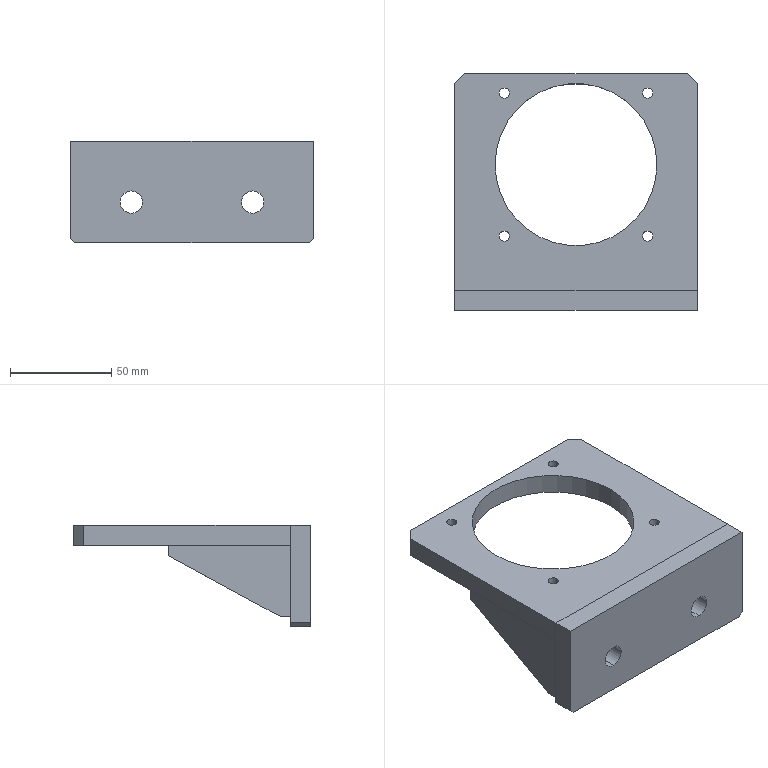Part | SolidWorks | features ICE 3, Chamfer 2, HoleWzd 2, Extrusion 1, MirrorSolid 1 | 4 solids | 44 faces | box 120 x 117 x 50 mm | volume 147908 mm3 | plane 30 | cylinder 14 | commonest cylinder face diameters 5 x8 11 x4 80 x2
STEP:
#1=CARTESIAN_POINT('',(-60.,5.,15.));
#2=VERTEX_POINT('',#1);
#3=CARTESIAN_POINT('',(-60.,65.,15.));
#4=VERTEX_POINT('',#3);
#5=CARTESIAN_POINT('',(-60.,5.,15.));
#6=DIRECTION('',(0.,1.,0.));
#7=VECTOR('',#6,1000.);
#8=LINE('',#5,#7);
#9=EDGE_CURVE('',#2,#4,#8,.T.);
#10=ORIENTED_EDGE('',*,*,#9,.F.);
#11=CARTESIAN_POINT('',(-55.,5.,15.));
#12=VERTEX_POINT('',#11);
#13=CARTESIAN_POINT('',(-55.,5.,15.));
#14=DIRECTION('',(-1.,0.,0.));
#15=VECTOR('',#14,1000.);
#16=LINE('',#13,#15);
#17=EDGE_CURVE('',#12,#2,#16,.T.);
#18=ORIENTED_EDGE('',*,*,#17,.F.);
#19=CARTESIAN_POINT('',(-55.,65.,15.));
#20=VERTEX_POINT('',#19);
#21=CARTESIAN_POINT('',(-55.,5.,15.));
#22=DIRECTION('',(0.,1.,0.));
#23=VECTOR('',#22,1000.);
#24=LINE('',#21,#23);
#25=EDGE_CURVE('',#12,#20,#24,.T.);
#26=ORIENTED_EDGE('',*,*,#25,.T.);
#27=CARTESIAN_POINT('',(-55.,65.,15.));
#28=DIRECTION('',(-1.,0.,0.));
#29=VECTOR('',#28,1000.);
#30=LINE('',#27,#29);
#31=EDGE_CURVE('',#20,#4,#30,.T.);
#32=ORIENTED_EDGE('',*,*,#31,.T.);
#33=EDGE_LOOP('',(#10,#18,#26,#32));
#34=FACE_OUTER_BOUND('',#33,.T.);
#35=CARTESIAN_POINT('',(-55.,5.,15.));
#36=DIRECTION('',(0.,0.,1.));
#37=DIRECTION('',(1.,0.,0.));
#38=AXIS2_PLACEMENT_3D('',#35,#36,#37);
#39=PLANE('',#38);
#40=ADVANCED_FACE('',(#34),#39,.T.);
#41=CARTESIAN_POINT('',(-60.,5.,-20.));
#42=VERTEX_POINT('',#41);
#43=CARTESIAN_POINT('',(-60.,5.,-20.));
#44=DIRECTION('',(0.,0.,1.));
#45=VECTOR('',#44,1000.);
#46=LINE('',#43,#45);
#47=EDGE_CURVE('',#42,#2,#46,.T.);
#48=ORIENTED_EDGE('',*,*,#47,.F.);
#49=CARTESIAN_POINT('',(-55.,5.,-20.));
#50=VERTEX_POINT('',#49);
#51=CARTESIAN_POINT('',(-55.,5.,-20.));
#52=DIRECTION('',(-1.,0.,0.));
#53=VECTOR('',#52,1000.);
#54=LINE('',#51,#53);
#55=EDGE_CURVE('',#50,#42,#54,.T.);
#56=ORIENTED_EDGE('',*,*,#55,.F.);
#57=CARTESIAN_POINT('',(-55.,5.,-20.));
#58=DIRECTION('',(0.,0.,1.));
#59=VECTOR('',#58,1000.);
#60=LINE('',#57,#59);
#61=EDGE_CURVE('',#50,#12,#60,.T.);
#62=ORIENTED_EDGE('',*,*,#61,.T.);
#63=ORIENTED_EDGE('',*,*,#17,.T.);
#64=EDGE_LOOP('',(#48,#56,#62,#63));
#65=FACE_OUTER_BOUND('',#64,.T.);
#66=CARTESIAN_POINT('',(-55.,5.,-20.));
#67=DIRECTION('',(0.,-1.,0.));
#68=DIRECTION('',(0.,0.,-1.));
#69=AXIS2_PLACEMENT_3D('',#66,#67,#68);
#70=PLANE('',#69);
#71=ADVANCED_FACE('',(#65),#70,.T.);
#72=CARTESIAN_POINT('',(-60.,10.,-20.));
#73=VERTEX_POINT('',#72);
#74=CARTESIAN_POINT('',(-60.,10.,-20.));
#75=DIRECTION('',(0.,-1.,0.));
#76=VECTOR('',#75,1000.);
#77=LINE('',#74,#76);
#78=EDGE_CURVE('',#73,#42,#77,.T.);
#79=ORIENTED_EDGE('',*,*,#78,.F.);
#80=CARTESIAN_POINT('',(-55.,10.,-20.));
#81=VERTEX_POINT('',#80);
#82=CARTESIAN_POINT('',(-55.,10.,-20.));
#83=DIRECTION('',(-1.,0.,0.));
#84=VECTOR('',#83,1000.);
#85=LINE('',#82,#84);
#86=EDGE_CURVE('',#81,#73,#85,.T.);
#87=ORIENTED_EDGE('',*,*,#86,.F.);
#88=CARTESIAN_POINT('',(-55.,10.,-20.));
#89=DIRECTION('',(0.,-1.,0.));
#90=VECTOR('',#89,1000.);
#91=LINE('',#88,#90);
#92=EDGE_CURVE('',#81,#50,#91,.T.);
#93=ORIENTED_EDGE('',*,*,#92,.T.);
#94=ORIENTED_EDGE('',*,*,#55,.T.);
#95=EDGE_LOOP('',(#79,#87,#93,#94));
#96=FACE_OUTER_BOUND('',#95,.T.);
#97=CARTESIAN_POINT('',(-55.,10.,-20.));
#98=DIRECTION('',(0.,0.,-1.));
#99=DIRECTION('',(-1.,0.,0.));
#100=AXIS2_PLACEMENT_3D('',#97,#98,#99);
#101=PLANE('',#100);
#102=ADVANCED_FACE('',(#96),#101,.T.);
#103=CARTESIAN_POINT('',(-60.,65.,10.));
#104=VERTEX_POINT('',#103);
#105=CARTESIAN_POINT('',(-60.,65.,10.));
#106=DIRECTION('',(0.,-0.8779,-0.4789));
#107=VECTOR('',#106,1000.);
#108=LINE('',#105,#107);
#109=EDGE_CURVE('',#104,#73,#108,.T.);
#110=ORIENTED_EDGE('',*,*,#109,.F.);
#111=CARTESIAN_POINT('',(-55.,65.,10.));
#112=VERTEX_POINT('',#111);
#113=CARTESIAN_POINT('',(-55.,65.,10.));
#114=DIRECTION('',(-1.,0.,0.));
#115=VECTOR('',#114,1000.);
#116=LINE('',#113,#115);
#117=EDGE_CURVE('',#112,#104,#116,.T.);
#118=ORIENTED_EDGE('',*,*,#117,.F.);
#119=CARTESIAN_POINT('',(-55.,65.,10.));
#120=DIRECTION('',(0.,-0.8779,-0.4789));
#121=VECTOR('',#120,1000.);
#122=LINE('',#119,#121);
#123=EDGE_CURVE('',#112,#81,#122,.T.);
#124=ORIENTED_EDGE('',*,*,#123,.T.);
#125=ORIENTED_EDGE('',*,*,#86,.T.);
#126=EDGE_LOOP('',(#110,#118,#124,#125));
#127=FACE_OUTER_BOUND('',#126,.T.);
#128=CARTESIAN_POINT('',(-55.,65.,10.));
#129=DIRECTION('',(0.,0.4789,-0.8779));
#130=DIRECTION('',(0.,0.8779,0.4789));
#131=AXIS2_PLACEMENT_3D('',#128,#129,#130);
#132=PLANE('',#131);
#133=ADVANCED_FACE('',(#127),#132,.T.);
#134=CARTESIAN_POINT('',(-60.,65.,15.));
#135=DIRECTION('',(0.,0.,-1.));
#136=VECTOR('',#135,1000.);
#137=LINE('',#134,#136);
#138=EDGE_CURVE('',#4,#104,#137,.T.);
#139=ORIENTED_EDGE('',*,*,#138,.F.);
#140=ORIENTED_EDGE('',*,*,#31,.F.);
#141=CARTESIAN_POINT('',(-55.,65.,15.));
#142=DIRECTION('',(0.,0.,-1.));
#143=VECTOR('',#142,1000.);
#144=LINE('',#141,#143);
#145=EDGE_CURVE('',#20,#112,#144,.T.);
#146=ORIENTED_EDGE('',*,*,#145,.T.);
#147=ORIENTED_EDGE('',*,*,#117,.T.);
#148=EDGE_LOOP('',(#139,#140,#146,#147));
#149=FACE_OUTER_BOUND('',#148,.T.);
#150=CARTESIAN_POINT('',(-55.,65.,15.));
#151=DIRECTION('',(0.,1.,0.));
#152=DIRECTION('',(0.,0.,1.));
#153=AXIS2_PLACEMENT_3D('',#150,#151,#152);
#154=PLANE('',#153);
#155=ADVANCED_FACE('',(#149),#154,.T.);
#156=ORIENTED_EDGE('',*,*,#25,.F.);
#157=ORIENTED_EDGE('',*,*,#61,.F.);
#158=ORIENTED_EDGE('',*,*,#92,.F.);
#159=ORIENTED_EDGE('',*,*,#123,.F.);
#160=ORIENTED_EDGE('',*,*,#145,.F.);
#161=EDGE_LOOP('',(#156,#157,#158,#159,#160));
#162=FACE_OUTER_BOUND('',#161,.T.);
#163=CARTESIAN_POINT('',(-55.,0.,0.));
#164=DIRECTION('',(-1.,0.,0.));
#165=DIRECTION('',(0.,0.,1.));
#166=AXIS2_PLACEMENT_3D('',#163,#164,#165);
#167=PLANE('',#166);
#168=ADVANCED_FACE('',(#162),#167,.F.);
#169=ORIENTED_EDGE('',*,*,#9,.T.);
#170=ORIENTED_EDGE('',*,*,#138,.T.);
#171=ORIENTED_EDGE('',*,*,#109,.T.);
#172=ORIENTED_EDGE('',*,*,#78,.T.);
#173=ORIENTED_EDGE('',*,*,#47,.T.);
#174=EDGE_LOOP('',(#169,#170,#171,#172,#173));
#175=FACE_OUTER_BOUND('',#174,.T.);
#176=CARTESIAN_POINT('',(-60.,0.,0.));
#177=DIRECTION('',(-1.,0.,0.));
#178=DIRECTION('',(0.,0.,1.));
#179=AXIS2_PLACEMENT_3D('',#176,#177,#178);
#180=PLANE('',#179);
#181=ADVANCED_FACE('',(#175),#180,.T.);
#182=CLOSED_SHELL('',(#40,#71,#102,#133,#155,#168,#181));
#183=MANIFOLD_SOLID_BREP('',#182);
#184=CARTESIAN_POINT('',(60.,5.,15.));
#185=VERTEX_POINT('',#184);
#186=CARTESIAN_POINT('',(60.,65.,15.));
#187=VERTEX_POINT('',#186);
#188=CARTESIAN_POINT('',(60.,5.,15.));
#189=DIRECTION('',(0.,1.,0.));
#190=VECTOR('',#189,1000.);
#191=LINE('',#188,#190);
#192=EDGE_CURVE('',#185,#187,#191,.T.);
#193=ORIENTED_EDGE('',*,*,#192,.T.);
#194=CARTESIAN_POINT('',(55.,65.,15.));
#195=VERTEX_POINT('',#194);
#196=CARTESIAN_POINT('',(55.,65.,15.));
#197=DIRECTION('',(1.,0.,0.));
#198=VECTOR('',#197,1000.);
#199=LINE('',#196,#198);
#200=EDGE_CURVE('',#195,#187,#199,.T.);
#201=ORIENTED_EDGE('',*,*,#200,.F.);
#202=CARTESIAN_POINT('',(55.,5.,15.));
#203=VERTEX_POINT('',#202);
#204=CARTESIAN_POINT('',(55.,5.,15.));
#205=DIRECTION('',(0.,1.,0.));
#206=VECTOR('',#205,1000.);
#207=LINE('',#204,#206);
#208=EDGE_CURVE('',#203,#195,#207,.T.);
#209=ORIENTED_EDGE('',*,*,#208,.F.);
#210=CARTESIAN_POINT('',(55.,5.,15.));
#211=DIRECTION('',(1.,0.,0.));
#212=VECTOR('',#211,1000.);
#213=LINE('',#210,#212);
#214=EDGE_CURVE('',#203,#185,#213,.T.);
#215=ORIENTED_EDGE('',*,*,#214,.T.);
#216=EDGE_LOOP('',(#193,#201,#209,#215));
#217=FACE_OUTER_BOUND('',#216,.T.);
#218=CARTESIAN_POINT('',(55.,5.,15.));
#219=DIRECTION('',(0.,0.,1.));
#220=DIRECTION('',(-1.,0.,0.));
#221=AXIS2_PLACEMENT_3D('',#218,#219,#220);
#222=PLANE('',#221);
#223=ADVANCED_FACE('',(#217),#222,.T.);
#224=CARTESIAN_POINT('',(60.,5.,-20.));
#225=VERTEX_POINT('',#224);
#226=CARTESIAN_POINT('',(60.,5.,-20.));
#227=DIRECTION('',(0.,0.,1.));
#228=VECTOR('',#227,1000.);
#229=LINE('',#226,#228);
#230=EDGE_CURVE('',#225,#185,#229,.T.);
#231=ORIENTED_EDGE('',*,*,#230,.T.);
#232=ORIENTED_EDGE('',*,*,#214,.F.);
#233=CARTESIAN_POINT('',(55.,5.,-20.));
#234=VERTEX_POINT('',#233);
#235=CARTESIAN_POINT('',(55.,5.,-20.));
#236=DIRECTION('',(0.,0.,1.));
#237=VECTOR('',#236,1000.);
#238=LINE('',#235,#237);
#239=EDGE_CURVE('',#234,#203,#238,.T.);
#240=ORIENTED_EDGE('',*,*,#239,.F.);
#241=CARTESIAN_POINT('',(55.,5.,-20.));
#242=DIRECTION('',(1.,0.,0.));
#243=VECTOR('',#242,1000.);
#244=LINE('',#241,#243);
#245=EDGE_CURVE('',#234,#225,#244,.T.);
#246=ORIENTED_EDGE('',*,*,#245,.T.);
#247=EDGE_LOOP('',(#231,#232,#240,#246));
#248=FACE_OUTER_BOUND('',#247,.T.);
#249=CARTESIAN_POINT('',(55.,5.,-20.));
#250=DIRECTION('',(0.,-1.,0.));
#251=DIRECTION('',(0.,0.,-1.));
#252=AXIS2_PLACEMENT_3D('',#249,#250,#251);
#253=PLANE('',#252);
#254=ADVANCED_FACE('',(#248),#253,.T.);
#255=CARTESIAN_POINT('',(60.,10.,-20.));
#256=VERTEX_POINT('',#255);
#257=CARTESIAN_POINT('',(60.,10.,-20.));
#258=DIRECTION('',(0.,-1.,0.));
#259=VECTOR('',#258,1000.);
#260=LINE('',#257,#259);
#261=EDGE_CURVE('',#256,#225,#260,.T.);
#262=ORIENTED_EDGE('',*,*,#261,.T.);
#263=ORIENTED_EDGE('',*,*,#245,.F.);
#264=CARTESIAN_POINT('',(55.,10.,-20.));
#265=VERTEX_POINT('',#264);
#266=CARTESIAN_POINT('',(55.,10.,-20.));
#267=DIRECTION('',(0.,-1.,0.));
#268=VECTOR('',#267,1000.);
#269=LINE('',#266,#268);
#270=EDGE_CURVE('',#265,#234,#269,.T.);
#271=ORIENTED_EDGE('',*,*,#270,.F.);
#272=CARTESIAN_POINT('',(55.,10.,-20.));
#273=DIRECTION('',(1.,0.,0.));
#274=VECTOR('',#273,1000.);
#275=LINE('',#272,#274);
#276=EDGE_CURVE('',#265,#256,#275,.T.);
#277=ORIENTED_EDGE('',*,*,#276,.T.);
#278=EDGE_LOOP('',(#262,#263,#271,#277));
#279=FACE_OUTER_BOUND('',#278,.T.);
#280=CARTESIAN_POINT('',(55.,10.,-20.));
#281=DIRECTION('',(0.,0.,-1.));
#282=DIRECTION('',(1.,0.,0.));
#283=AXIS2_PLACEMENT_3D('',#280,#281,#282);
#284=PLANE('',#283);
#285=ADVANCED_FACE('',(#279),#284,.T.);
#286=CARTESIAN_POINT('',(60.,65.,10.));
#287=VERTEX_POINT('',#286);
#288=CARTESIAN_POINT('',(60.,65.,10.));
#289=DIRECTION('',(0.,-0.8779,-0.4789));
#290=VECTOR('',#289,1000.);
#291=LINE('',#288,#290);
#292=EDGE_CURVE('',#287,#256,#291,.T.);
#293=ORIENTED_EDGE('',*,*,#292,.T.);
#294=ORIENTED_EDGE('',*,*,#276,.F.);
#295=CARTESIAN_POINT('',(55.,65.,10.));
#296=VERTEX_POINT('',#295);
#297=CARTESIAN_POINT('',(55.,65.,10.));
#298=DIRECTION('',(0.,-0.8779,-0.4789));
#299=VECTOR('',#298,1000.);
#300=LINE('',#297,#299);
#301=EDGE_CURVE('',#296,#265,#300,.T.);
#302=ORIENTED_EDGE('',*,*,#301,.F.);
#303=CARTESIAN_POINT('',(55.,65.,10.));
#304=DIRECTION('',(1.,0.,0.));
#305=VECTOR('',#304,1000.);
#306=LINE('',#303,#305);
#307=EDGE_CURVE('',#296,#287,#306,.T.);
#308=ORIENTED_EDGE('',*,*,#307,.T.);
#309=EDGE_LOOP('',(#293,#294,#302,#308));
#310=FACE_OUTER_BOUND('',#309,.T.);
#311=CARTESIAN_POINT('',(55.,65.,10.));
#312=DIRECTION('',(0.,0.4789,-0.8779));
#313=DIRECTION('',(0.,0.8779,0.4789));
#314=AXIS2_PLACEMENT_3D('',#311,#312,#313);
#315=PLANE('',#314);
#316=ADVANCED_FACE('',(#310),#315,.T.);
#317=CARTESIAN_POINT('',(60.,65.,15.));
#318=DIRECTION('',(0.,0.,-1.));
#319=VECTOR('',#318,1000.);
#320=LINE('',#317,#319);
#321=EDGE_CURVE('',#187,#287,#320,.T.);
#322=ORIENTED_EDGE('',*,*,#321,.T.);
#323=ORIENTED_EDGE('',*,*,#307,.F.);
#324=CARTESIAN_POINT('',(55.,65.,15.));
#325=DIRECTION('',(0.,0.,-1.));
#326=VECTOR('',#325,1000.);
#327=LINE('',#324,#326);
#328=EDGE_CURVE('',#195,#296,#327,.T.);
#329=ORIENTED_EDGE('',*,*,#328,.F.);
#330=ORIENTED_EDGE('',*,*,#200,.T.);
#331=EDGE_LOOP('',(#322,#323,#329,#330));
#332=FACE_OUTER_BOUND('',#331,.T.);
#333=CARTESIAN_POINT('',(55.,65.,15.));
#334=DIRECTION('',(0.,1.,0.));
#335=DIRECTION('',(0.,0.,1.));
#336=AXIS2_PLACEMENT_3D('',#333,#334,#335);
#337=PLANE('',#336);
#338=ADVANCED_FACE('',(#332),#337,.T.);
#339=ORIENTED_EDGE('',*,*,#208,.T.);
#340=ORIENTED_EDGE('',*,*,#328,.T.);
#341=ORIENTED_EDGE('',*,*,#301,.T.);
#342=ORIENTED_EDGE('',*,*,#270,.T.);
#343=ORIENTED_EDGE('',*,*,#239,.T.);
#344=EDGE_LOOP('',(#339,#340,#341,#342,#343));
#345=FACE_OUTER_BOUND('',#344,.T.);
#346=CARTESIAN_POINT('',(55.,0.,0.));
#347=DIRECTION('',(1.,0.,0.));
#348=DIRECTION('',(0.,0.,1.));
#349=AXIS2_PLACEMENT_3D('',#346,#347,#348);
#350=PLANE('',#349);
#351=ADVANCED_FACE('',(#345),#350,.F.);
#352=ORIENTED_EDGE('',*,*,#192,.F.);
#353=ORIENTED_EDGE('',*,*,#230,.F.);
#354=ORIENTED_EDGE('',*,*,#261,.F.);
#355=ORIENTED_EDGE('',*,*,#292,.F.);
#356=ORIENTED_EDGE('',*,*,#321,.F.);
#357=EDGE_LOOP('',(#352,#353,#354,#355,#356));
#358=FACE_OUTER_BOUND('',#357,.T.);
#359=CARTESIAN_POINT('',(60.,0.,0.));
#360=DIRECTION('',(1.,0.,0.));
#361=DIRECTION('',(0.,0.,1.));
#362=AXIS2_PLACEMENT_3D('',#359,#360,#361);
#363=PLANE('',#362);
#364=ADVANCED_FACE('',(#358),#363,.T.);
#365=CLOSED_SHELL('',(#223,#254,#285,#316,#338,#351,#364));
#366=MANIFOLD_SOLID_BREP('',#365);
#367=CARTESIAN_POINT('',(30.,-5.,-10.5));
#368=VERTEX_POINT('',#367);
#369=CARTESIAN_POINT('',(30.,-5.,0.5));
#370=VERTEX_POINT('',#369);
#371=CARTESIAN_POINT('',(30.,-5.,-5.));
#372=DIRECTION('',(0.,1.,0.));
#373=DIRECTION('',(0.,0.,1.));
#374=AXIS2_PLACEMENT_3D('',#371,#372,#373);
#375=CIRCLE('',#374,5.5);
#376=EDGE_CURVE('',#368,#370,#375,.T.);
#377=ORIENTED_EDGE('',*,*,#376,.F.);
#378=CARTESIAN_POINT('',(30.,5.,-10.5));
#379=VERTEX_POINT('',#378);
#380=CARTESIAN_POINT('',(30.,5.,-10.5));
#381=DIRECTION('',(0.,1.,0.));
#382=VECTOR('',#381,1000.);
#383=LINE('',#380,#382);
#384=EDGE_CURVE('',#368,#379,#383,.T.);
#385=ORIENTED_EDGE('',*,*,#384,.T.);
#386=CARTESIAN_POINT('',(30.,5.,0.5));
#387=VERTEX_POINT('',#386);
#388=CARTESIAN_POINT('',(30.,5.,-5.));
#389=DIRECTION('',(0.,1.,0.));
#390=DIRECTION('',(0.,0.,1.));
#391=AXIS2_PLACEMENT_3D('',#388,#389,#390);
#392=CIRCLE('',#391,5.5);
#393=EDGE_CURVE('',#379,#387,#392,.T.);
#394=ORIENTED_EDGE('',*,*,#393,.T.);
#395=CARTESIAN_POINT('',(30.,5.,0.5));
#396=DIRECTION('',(0.,1.,0.));
#397=VECTOR('',#396,1000.);
#398=LINE('',#395,#397);
#399=EDGE_CURVE('',#370,#387,#398,.T.);
#400=ORIENTED_EDGE('',*,*,#399,.F.);
#401=EDGE_LOOP('',(#377,#385,#394,#400));
#402=FACE_OUTER_BOUND('',#401,.T.);
#403=CARTESIAN_POINT('',(30.,5.,-5.));
#404=DIRECTION('',(0.,1.,0.));
#405=DIRECTION('',(0.,0.,1.));
#406=AXIS2_PLACEMENT_3D('',#403,#404,#405);
#407=CYLINDRICAL_SURFACE('',#406,5.5);
#408=ADVANCED_FACE('',(#402),#407,.F.);
#409=CARTESIAN_POINT('',(-30.,-5.,-10.5));
#410=VERTEX_POINT('',#409);
#411=CARTESIAN_POINT('',(-30.,-5.,0.5));
#412=VERTEX_POINT('',#411);
#413=CARTESIAN_POINT('',(-30.,-5.,-5.));
#414=DIRECTION('',(0.,1.,0.));
#415=DIRECTION('',(0.,0.,1.));
#416=AXIS2_PLACEMENT_3D('',#413,#414,#415);
#417=CIRCLE('',#416,5.5);
#418=EDGE_CURVE('',#410,#412,#417,.T.);
#419=ORIENTED_EDGE('',*,*,#418,.F.);
#420=CARTESIAN_POINT('',(-30.,5.,-10.5));
#421=VERTEX_POINT('',#420);
#422=CARTESIAN_POINT('',(-30.,5.,-10.5));
#423=DIRECTION('',(0.,1.,0.));
#424=VECTOR('',#423,1000.);
#425=LINE('',#422,#424);
#426=EDGE_CURVE('',#410,#421,#425,.T.);
#427=ORIENTED_EDGE('',*,*,#426,.T.);
#428=CARTESIAN_POINT('',(-30.,5.,0.5));
#429=VERTEX_POINT('',#428);
#430=CARTESIAN_POINT('',(-30.,5.,-5.));
#431=DIRECTION('',(0.,1.,0.));
#432=DIRECTION('',(0.,0.,1.));
#433=AXIS2_PLACEMENT_3D('',#430,#431,#432);
#434=CIRCLE('',#433,5.5);
#435=EDGE_CURVE('',#421,#429,#434,.T.);
#436=ORIENTED_EDGE('',*,*,#435,.T.);
#437=CARTESIAN_POINT('',(-30.,5.,0.5));
#438=DIRECTION('',(0.,1.,0.));
#439=VECTOR('',#438,1000.);
#440=LINE('',#437,#439);
#441=EDGE_CURVE('',#412,#429,#440,.T.);
#442=ORIENTED_EDGE('',*,*,#441,.F.);
#443=EDGE_LOOP('',(#419,#427,#436,#442));
#444=FACE_OUTER_BOUND('',#443,.T.);
#445=CARTESIAN_POINT('',(-30.,5.,-5.));
#446=DIRECTION('',(0.,1.,0.));
#447=DIRECTION('',(0.,0.,1.));
#448=AXIS2_PLACEMENT_3D('',#445,#446,#447);
#449=CYLINDRICAL_SURFACE('',#448,5.5);
#450=ADVANCED_FACE('',(#444),#449,.F.);
#451=CARTESIAN_POINT('',(60.,-5.,25.));
#452=VERTEX_POINT('',#451);
#453=CARTESIAN_POINT('',(60.,-5.,-23.));
#454=VERTEX_POINT('',#453);
#455=CARTESIAN_POINT('',(60.,-5.,25.));
#456=DIRECTION('',(0.,0.,-1.));
#457=VECTOR('',#456,1000.);
#458=LINE('',#455,#457);
#459=EDGE_CURVE('',#452,#454,#458,.T.);
#460=ORIENTED_EDGE('',*,*,#459,.T.);
#461=CARTESIAN_POINT('',(60.,5.,-23.));
#462=VERTEX_POINT('',#461);
#463=CARTESIAN_POINT('',(60.,5.,-23.));
#464=DIRECTION('',(0.,1.,0.));
#465=VECTOR('',#464,1000.);
#466=LINE('',#463,#465);
#467=EDGE_CURVE('',#454,#462,#466,.T.);
#468=ORIENTED_EDGE('',*,*,#467,.T.);
#469=CARTESIAN_POINT('',(60.,5.,25.));
#470=VERTEX_POINT('',#469);
#471=CARTESIAN_POINT('',(60.,5.,25.));
#472=DIRECTION('',(0.,0.,-1.));
#473=VECTOR('',#472,1000.);
#474=LINE('',#471,#473);
#475=EDGE_CURVE('',#470,#462,#474,.T.);
#476=ORIENTED_EDGE('',*,*,#475,.F.);
#477=CARTESIAN_POINT('',(60.,5.,25.));
#478=DIRECTION('',(0.,-1.,0.));
#479=VECTOR('',#478,1000.);
#480=LINE('',#477,#479);
#481=EDGE_CURVE('',#470,#452,#480,.T.);
#482=ORIENTED_EDGE('',*,*,#481,.T.);
#483=EDGE_LOOP('',(#460,#468,#476,#482));
#484=FACE_OUTER_BOUND('',#483,.T.);
#485=CARTESIAN_POINT('',(60.,5.,25.));
#486=DIRECTION('',(-1.,0.,0.));
#487=DIRECTION('',(0.,0.,1.));
#488=AXIS2_PLACEMENT_3D('',#485,#486,#487);
#489=PLANE('',#488);
#490=ADVANCED_FACE('',(#484),#489,.F.);
#491=CARTESIAN_POINT('',(58.,-5.,-25.));
#492=VERTEX_POINT('',#491);
#493=CARTESIAN_POINT('',(-58.,-5.,-25.));
#494=VERTEX_POINT('',#493);
#495=CARTESIAN_POINT('',(-60.,-5.,-25.));
#496=DIRECTION('',(-1.,0.,0.));
#497=VECTOR('',#496,1000.);
#498=LINE('',#495,#497);
#499=EDGE_CURVE('',#492,#494,#498,.T.);
#500=ORIENTED_EDGE('',*,*,#499,.T.);
#501=CARTESIAN_POINT('',(-58.,5.,-25.));
#502=VERTEX_POINT('',#501);
#503=CARTESIAN_POINT('',(-58.,5.,-25.));
#504=DIRECTION('',(0.,1.,0.));
#505=VECTOR('',#504,1000.);
#506=LINE('',#503,#505);
#507=EDGE_CURVE('',#494,#502,#506,.T.);
#508=ORIENTED_EDGE('',*,*,#507,.T.);
#509=CARTESIAN_POINT('',(58.,5.,-25.));
#510=VERTEX_POINT('',#509);
#511=CARTESIAN_POINT('',(-60.,5.,-25.));
#512=DIRECTION('',(-1.,0.,0.));
#513=VECTOR('',#512,1000.);
#514=LINE('',#511,#513);
#515=EDGE_CURVE('',#510,#502,#514,.T.);
#516=ORIENTED_EDGE('',*,*,#515,.F.);
#517=CARTESIAN_POINT('',(58.,5.,-25.));
#518=DIRECTION('',(0.,-1.,0.));
#519=VECTOR('',#518,1000.);
#520=LINE('',#517,#519);
#521=EDGE_CURVE('',#510,#492,#520,.T.);
#522=ORIENTED_EDGE('',*,*,#521,.T.);
#523=EDGE_LOOP('',(#500,#508,#516,#522));
#524=FACE_OUTER_BOUND('',#523,.T.);
#525=CARTESIAN_POINT('',(-60.,5.,-25.));
#526=DIRECTION('',(0.,0.,1.));
#527=DIRECTION('',(1.,0.,0.));
#528=AXIS2_PLACEMENT_3D('',#525,#526,#527);
#529=PLANE('',#528);
#530=ADVANCED_FACE('',(#524),#529,.F.);
#531=CARTESIAN_POINT('',(-60.,5.,-23.));
#532=VERTEX_POINT('',#531);
#533=CARTESIAN_POINT('',(-60.,5.,25.));
#534=VERTEX_POINT('',#533);
#535=CARTESIAN_POINT('',(-60.,5.,25.));
#536=DIRECTION('',(0.,0.,1.));
#537=VECTOR('',#536,1000.);
#538=LINE('',#535,#537);
#539=EDGE_CURVE('',#532,#534,#538,.T.);
#540=ORIENTED_EDGE('',*,*,#539,.F.);
#541=CARTESIAN_POINT('',(-60.,-5.,-23.));
#542=VERTEX_POINT('',#541);
#543=CARTESIAN_POINT('',(-60.,5.,-23.));
#544=DIRECTION('',(0.,-1.,0.));
#545=VECTOR('',#544,1000.);
#546=LINE('',#543,#545);
#547=EDGE_CURVE('',#532,#542,#546,.T.);
#548=ORIENTED_EDGE('',*,*,#547,.T.);
#549=CARTESIAN_POINT('',(-60.,-5.,25.));
#550=VERTEX_POINT('',#549);
#551=CARTESIAN_POINT('',(-60.,-5.,25.));
#552=DIRECTION('',(0.,0.,1.));
#553=VECTOR('',#552,1000.);
#554=LINE('',#551,#553);
#555=EDGE_CURVE('',#542,#550,#554,.T.);
#556=ORIENTED_EDGE('',*,*,#555,.T.);
#557=CARTESIAN_POINT('',(-60.,5.,25.));
#558=DIRECTION('',(0.,-1.,0.));
#559=VECTOR('',#558,1000.);
#560=LINE('',#557,#559);
#561=EDGE_CURVE('',#534,#550,#560,.T.);
#562=ORIENTED_EDGE('',*,*,#561,.F.);
#563=EDGE_LOOP('',(#540,#548,#556,#562));
#564=FACE_OUTER_BOUND('',#563,.T.);
#565=CARTESIAN_POINT('',(-60.,5.,25.));
#566=DIRECTION('',(1.,0.,0.));
#567=DIRECTION('',(0.,0.,-1.));
#568=AXIS2_PLACEMENT_3D('',#565,#566,#567);
#569=PLANE('',#568);
#570=ADVANCED_FACE('',(#564),#569,.F.);
#571=CARTESIAN_POINT('',(-60.,-5.,25.));
#572=DIRECTION('',(1.,0.,0.));
#573=VECTOR('',#572,1000.);
#574=LINE('',#571,#573);
#575=EDGE_CURVE('',#550,#452,#574,.T.);
#576=ORIENTED_EDGE('',*,*,#575,.T.);
#577=ORIENTED_EDGE('',*,*,#481,.F.);
#578=CARTESIAN_POINT('',(-60.,5.,25.));
#579=DIRECTION('',(1.,0.,0.));
#580=VECTOR('',#579,1000.);
#581=LINE('',#578,#580);
#582=EDGE_CURVE('',#534,#470,#581,.T.);
#583=ORIENTED_EDGE('',*,*,#582,.F.);
#584=ORIENTED_EDGE('',*,*,#561,.T.);
#585=EDGE_LOOP('',(#576,#577,#583,#584));
#586=FACE_OUTER_BOUND('',#585,.T.);
#587=CARTESIAN_POINT('',(-60.,5.,25.));
#588=DIRECTION('',(0.,0.,-1.));
#589=DIRECTION('',(-1.,0.,0.));
#590=AXIS2_PLACEMENT_3D('',#587,#588,#589);
#591=PLANE('',#590);
#592=ADVANCED_FACE('',(#586),#591,.F.);
#593=CARTESIAN_POINT('',(30.,5.,-5.));
#594=DIRECTION('',(0.,1.,0.));
#595=DIRECTION('',(0.,0.,1.));
#596=AXIS2_PLACEMENT_3D('',#593,#594,#595);
#597=CIRCLE('',#596,5.5);
#598=EDGE_CURVE('',#387,#379,#597,.T.);
#599=ORIENTED_EDGE('',*,*,#598,.F.);
#600=ORIENTED_EDGE('',*,*,#393,.F.);
#601=EDGE_LOOP('',(#599,#600));
#602=FACE_BOUND('',#601,.T.);
#603=CARTESIAN_POINT('',(-30.,5.,-5.));
#604=DIRECTION('',(0.,1.,0.));
#605=DIRECTION('',(0.,0.,1.));
#606=AXIS2_PLACEMENT_3D('',#603,#604,#605);
#607=CIRCLE('',#606,5.5);
#608=EDGE_CURVE('',#429,#421,#607,.T.);
#609=ORIENTED_EDGE('',*,*,#608,.F.);
#610=ORIENTED_EDGE('',*,*,#435,.F.);
#611=EDGE_LOOP('',(#609,#610));
#612=FACE_BOUND('',#611,.T.);
#613=ORIENTED_EDGE('',*,*,#515,.T.);
#614=CARTESIAN_POINT('',(-60.,5.,-23.));
#615=DIRECTION('',(-0.7071,0.,0.7071));
#616=VECTOR('',#615,1000.);
#617=LINE('',#614,#616);
#618=EDGE_CURVE('',#502,#532,#617,.T.);
#619=ORIENTED_EDGE('',*,*,#618,.T.);
#620=ORIENTED_EDGE('',*,*,#539,.T.);
#621=ORIENTED_EDGE('',*,*,#582,.T.);
#622=ORIENTED_EDGE('',*,*,#475,.T.);
#623=CARTESIAN_POINT('',(58.,5.,-25.));
#624=DIRECTION('',(-0.7071,0.,-0.7071));
#625=VECTOR('',#624,1000.);
#626=LINE('',#623,#625);
#627=EDGE_CURVE('',#462,#510,#626,.T.);
#628=ORIENTED_EDGE('',*,*,#627,.T.);
#629=EDGE_LOOP('',(#613,#619,#620,#621,#622,#628));
#630=FACE_OUTER_BOUND('',#629,.T.);
#631=CARTESIAN_POINT('',(0.,5.,0.));
#632=DIRECTION('',(0.,-1.,0.));
#633=DIRECTION('',(0.,0.,-1.));
#634=AXIS2_PLACEMENT_3D('',#631,#632,#633);
#635=PLANE('',#634);
#636=ADVANCED_FACE('',(#602,#612,#630),#635,.F.);
#637=CARTESIAN_POINT('',(30.,-5.,-5.));
#638=DIRECTION('',(0.,1.,0.));
#639=DIRECTION('',(0.,0.,1.));
#640=AXIS2_PLACEMENT_3D('',#637,#638,#639);
#641=CIRCLE('',#640,5.5);
#642=EDGE_CURVE('',#370,#368,#641,.T.);
#643=ORIENTED_EDGE('',*,*,#642,.T.);
#644=ORIENTED_EDGE('',*,*,#376,.T.);
#645=EDGE_LOOP('',(#643,#644));
#646=FACE_BOUND('',#645,.T.);
#647=CARTESIAN_POINT('',(-30.,-5.,-5.));
#648=DIRECTION('',(0.,1.,0.));
#649=DIRECTION('',(0.,0.,1.));
#650=AXIS2_PLACEMENT_3D('',#647,#648,#649);
#651=CIRCLE('',#650,5.5);
#652=EDGE_CURVE('',#412,#410,#651,.T.);
#653=ORIENTED_EDGE('',*,*,#652,.T.);
#654=ORIENTED_EDGE('',*,*,#418,.T.);
#655=EDGE_LOOP('',(#653,#654));
#656=FACE_BOUND('',#655,.T.);
#657=ORIENTED_EDGE('',*,*,#555,.F.);
#658=CARTESIAN_POINT('',(-41.5,-5.,-41.5));
#659=DIRECTION('',(0.7071,0.,-0.7071));
#660=VECTOR('',#659,1000.);
#661=LINE('',#658,#660);
#662=EDGE_CURVE('',#542,#494,#661,.T.);
#663=ORIENTED_EDGE('',*,*,#662,.T.);
#664=ORIENTED_EDGE('',*,*,#499,.F.);
#665=CARTESIAN_POINT('',(41.5,-5.,-41.5));
#666=DIRECTION('',(0.7071,0.,0.7071));
#667=VECTOR('',#666,1000.);
#668=LINE('',#665,#667);
#669=EDGE_CURVE('',#492,#454,#668,.T.);
#670=ORIENTED_EDGE('',*,*,#669,.T.);
#671=ORIENTED_EDGE('',*,*,#459,.F.);
#672=ORIENTED_EDGE('',*,*,#575,.F.);
#673=EDGE_LOOP('',(#657,#663,#664,#670,#671,#672));
#674=FACE_OUTER_BOUND('',#673,.T.);
#675=CARTESIAN_POINT('',(0.,-5.,0.));
#676=DIRECTION('',(0.,-1.,0.));
#677=DIRECTION('',(0.,0.,-1.));
#678=AXIS2_PLACEMENT_3D('',#675,#676,#677);
#679=PLANE('',#678);
#680=ADVANCED_FACE('',(#646,#656,#674),#679,.T.);
#681=ORIENTED_EDGE('',*,*,#618,.F.);
#682=ORIENTED_EDGE('',*,*,#507,.F.);
#683=ORIENTED_EDGE('',*,*,#662,.F.);
#684=ORIENTED_EDGE('',*,*,#547,.F.);
#685=EDGE_LOOP('',(#681,#682,#683,#684));
#686=FACE_OUTER_BOUND('',#685,.T.);
#687=CARTESIAN_POINT('',(-60.,5.,-23.));
#688=DIRECTION('',(0.7071,0.,0.7071));
#689=DIRECTION('',(0.,-1.,0.));
#690=AXIS2_PLACEMENT_3D('',#687,#688,#689);
#691=PLANE('',#690);
#692=ADVANCED_FACE('',(#686),#691,.F.);
#693=ORIENTED_EDGE('',*,*,#627,.F.);
#694=ORIENTED_EDGE('',*,*,#467,.F.);
#695=ORIENTED_EDGE('',*,*,#669,.F.);
#696=ORIENTED_EDGE('',*,*,#521,.F.);
#697=EDGE_LOOP('',(#693,#694,#695,#696));
#698=FACE_OUTER_BOUND('',#697,.T.);
#699=CARTESIAN_POINT('',(58.,5.,-25.));
#700=DIRECTION('',(-0.7071,0.,0.7071));
#701=DIRECTION('',(0.,-1.,0.));
#702=AXIS2_PLACEMENT_3D('',#699,#700,#701);
#703=PLANE('',#702);
#704=ADVANCED_FACE('',(#698),#703,.F.);
#705=ORIENTED_EDGE('',*,*,#426,.F.);
#706=ORIENTED_EDGE('',*,*,#652,.F.);
#707=ORIENTED_EDGE('',*,*,#441,.T.);
#708=ORIENTED_EDGE('',*,*,#608,.T.);
#709=EDGE_LOOP('',(#705,#706,#707,#708));
#710=FACE_OUTER_BOUND('',#709,.T.);
#711=CARTESIAN_POINT('',(-30.,5.,-5.));
#712=DIRECTION('',(0.,1.,0.));
#713=DIRECTION('',(0.,0.,1.));
#714=AXIS2_PLACEMENT_3D('',#711,#712,#713);
#715=CYLINDRICAL_SURFACE('',#714,5.5);
#716=ADVANCED_FACE('',(#710),#715,.F.);
#717=ORIENTED_EDGE('',*,*,#384,.F.);
#718=ORIENTED_EDGE('',*,*,#642,.F.);
#719=ORIENTED_EDGE('',*,*,#399,.T.);
#720=ORIENTED_EDGE('',*,*,#598,.T.);
#721=EDGE_LOOP('',(#717,#718,#719,#720));
#722=FACE_OUTER_BOUND('',#721,.T.);
#723=CARTESIAN_POINT('',(30.,5.,-5.));
#724=DIRECTION('',(0.,1.,0.));
#725=DIRECTION('',(0.,0.,1.));
#726=AXIS2_PLACEMENT_3D('',#723,#724,#725);
#727=CYLINDRICAL_SURFACE('',#726,5.5);
#728=ADVANCED_FACE('',(#722),#727,.F.);
#729=CLOSED_SHELL('',(#408,#450,#490,#530,#570,#592,#636,#680,#692,#704,#716,#728));
#730=MANIFOLD_SOLID_BREP('',#729);
#731=CARTESIAN_POINT('',(-37.855,102.355,15.));
#732=VERTEX_POINT('',#731);
#733=CARTESIAN_POINT('',(-32.855,102.355,15.));
#734=VERTEX_POINT('',#733);
#735=CARTESIAN_POINT('',(-35.355,102.355,15.));
#736=DIRECTION('',(0.,0.,1.));
#737=DIRECTION('',(1.,0.,0.));
#738=AXIS2_PLACEMENT_3D('',#735,#736,#737);
#739=CIRCLE('',#738,2.5);
#740=EDGE_CURVE('',#732,#734,#739,.T.);
#741=ORIENTED_EDGE('',*,*,#740,.F.);
#742=CARTESIAN_POINT('',(-37.855,102.355,25.));
#743=VERTEX_POINT('',#742);
#744=CARTESIAN_POINT('',(-37.855,102.355,25.));
#745=DIRECTION('',(0.,0.,1.));
#746=VECTOR('',#745,1000.);
#747=LINE('',#744,#746);
#748=EDGE_CURVE('',#732,#743,#747,.T.);
#749=ORIENTED_EDGE('',*,*,#748,.T.);
#750=CARTESIAN_POINT('',(-32.855,102.355,25.));
#751=VERTEX_POINT('',#750);
#752=CARTESIAN_POINT('',(-35.355,102.355,25.));
#753=DIRECTION('',(0.,0.,1.));
#754=DIRECTION('',(1.,0.,0.));
#755=AXIS2_PLACEMENT_3D('',#752,#753,#754);
#756=CIRCLE('',#755,2.5);
#757=EDGE_CURVE('',#743,#751,#756,.T.);
#758=ORIENTED_EDGE('',*,*,#757,.T.);
#759=CARTESIAN_POINT('',(-32.855,102.355,25.));
#760=DIRECTION('',(0.,0.,1.));
#761=VECTOR('',#760,1000.);
#762=LINE('',#759,#761);
#763=EDGE_CURVE('',#734,#751,#762,.T.);
#764=ORIENTED_EDGE('',*,*,#763,.F.);
#765=EDGE_LOOP('',(#741,#749,#758,#764));
#766=FACE_OUTER_BOUND('',#765,.T.);
#767=CARTESIAN_POINT('',(-35.355,102.355,25.));
#768=DIRECTION('',(0.,0.,1.));
#769=DIRECTION('',(1.,0.,0.));
#770=AXIS2_PLACEMENT_3D('',#767,#768,#769);
#771=CYLINDRICAL_SURFACE('',#770,2.5);
#772=ADVANCED_FACE('',(#766),#771,.F.);
#773=CARTESIAN_POINT('',(32.855,102.355,15.));
#774=VERTEX_POINT('',#773);
#775=CARTESIAN_POINT('',(37.855,102.355,15.));
#776=VERTEX_POINT('',#775);
#777=CARTESIAN_POINT('',(35.355,102.355,15.));
#778=DIRECTION('',(0.,0.,1.));
#779=DIRECTION('',(1.,0.,0.));
#780=AXIS2_PLACEMENT_3D('',#777,#778,#779);
#781=CIRCLE('',#780,2.5);
#782=EDGE_CURVE('',#774,#776,#781,.T.);
#783=ORIENTED_EDGE('',*,*,#782,.F.);
#784=CARTESIAN_POINT('',(32.855,102.355,25.));
#785=VERTEX_POINT('',#784);
#786=CARTESIAN_POINT('',(32.855,102.355,25.));
#787=DIRECTION('',(0.,0.,1.));
#788=VECTOR('',#787,1000.);
#789=LINE('',#786,#788);
#790=EDGE_CURVE('',#774,#785,#789,.T.);
#791=ORIENTED_EDGE('',*,*,#790,.T.);
#792=CARTESIAN_POINT('',(37.855,102.355,25.));
#793=VERTEX_POINT('',#792);
#794=CARTESIAN_POINT('',(35.355,102.355,25.));
#795=DIRECTION('',(0.,0.,1.));
#796=DIRECTION('',(1.,0.,0.));
#797=AXIS2_PLACEMENT_3D('',#794,#795,#796);
#798=CIRCLE('',#797,2.5);
#799=EDGE_CURVE('',#785,#793,#798,.T.);
#800=ORIENTED_EDGE('',*,*,#799,.T.);
#801=CARTESIAN_POINT('',(37.855,102.355,25.));
#802=DIRECTION('',(0.,0.,1.));
#803=VECTOR('',#802,1000.);
#804=LINE('',#801,#803);
#805=EDGE_CURVE('',#776,#793,#804,.T.);
#806=ORIENTED_EDGE('',*,*,#805,.F.);
#807=EDGE_LOOP('',(#783,#791,#800,#806));
#808=FACE_OUTER_BOUND('',#807,.T.);
#809=CARTESIAN_POINT('',(35.355,102.355,25.));
#810=DIRECTION('',(0.,0.,1.));
#811=DIRECTION('',(1.,0.,0.));
#812=AXIS2_PLACEMENT_3D('',#809,#810,#811);
#813=CYLINDRICAL_SURFACE('',#812,2.5);
#814=ADVANCED_FACE('',(#808),#813,.F.);
#815=CARTESIAN_POINT('',(32.855,31.645,15.));
#816=VERTEX_POINT('',#815);
#817=CARTESIAN_POINT('',(37.855,31.645,15.));
#818=VERTEX_POINT('',#817);
#819=CARTESIAN_POINT('',(35.355,31.645,15.));
#820=DIRECTION('',(0.,0.,1.));
#821=DIRECTION('',(1.,0.,0.));
#822=AXIS2_PLACEMENT_3D('',#819,#820,#821);
#823=CIRCLE('',#822,2.5);
#824=EDGE_CURVE('',#816,#818,#823,.T.);
#825=ORIENTED_EDGE('',*,*,#824,.F.);
#826=CARTESIAN_POINT('',(32.855,31.645,25.));
#827=VERTEX_POINT('',#826);
#828=CARTESIAN_POINT('',(32.855,31.645,25.));
#829=DIRECTION('',(0.,0.,1.));
#830=VECTOR('',#829,1000.);
#831=LINE('',#828,#830);
#832=EDGE_CURVE('',#816,#827,#831,.T.);
#833=ORIENTED_EDGE('',*,*,#832,.T.);
#834=CARTESIAN_POINT('',(37.855,31.645,25.));
#835=VERTEX_POINT('',#834);
#836=CARTESIAN_POINT('',(35.355,31.645,25.));
#837=DIRECTION('',(0.,0.,1.));
#838=DIRECTION('',(1.,0.,0.));
#839=AXIS2_PLACEMENT_3D('',#836,#837,#838);
#840=CIRCLE('',#839,2.5);
#841=EDGE_CURVE('',#827,#835,#840,.T.);
#842=ORIENTED_EDGE('',*,*,#841,.T.);
#843=CARTESIAN_POINT('',(37.855,31.645,25.));
#844=DIRECTION('',(0.,0.,1.));
#845=VECTOR('',#844,1000.);
#846=LINE('',#843,#845);
#847=EDGE_CURVE('',#818,#835,#846,.T.);
#848=ORIENTED_EDGE('',*,*,#847,.F.);
#849=EDGE_LOOP('',(#825,#833,#842,#848));
#850=FACE_OUTER_BOUND('',#849,.T.);
#851=CARTESIAN_POINT('',(35.355,31.645,25.));
#852=DIRECTION('',(0.,0.,1.));
#853=DIRECTION('',(1.,0.,0.));
#854=AXIS2_PLACEMENT_3D('',#851,#852,#853);
#855=CYLINDRICAL_SURFACE('',#854,2.5);
#856=ADVANCED_FACE('',(#850),#855,.F.);
#857=CARTESIAN_POINT('',(-37.855,31.645,15.));
#858=VERTEX_POINT('',#857);
#859=CARTESIAN_POINT('',(-32.855,31.645,15.));
#860=VERTEX_POINT('',#859);
#861=CARTESIAN_POINT('',(-35.355,31.645,15.));
#862=DIRECTION('',(0.,0.,1.));
#863=DIRECTION('',(1.,0.,0.));
#864=AXIS2_PLACEMENT_3D('',#861,#862,#863);
#865=CIRCLE('',#864,2.5);
#866=EDGE_CURVE('',#858,#860,#865,.T.);
#867=ORIENTED_EDGE('',*,*,#866,.F.);
#868=CARTESIAN_POINT('',(-37.855,31.645,25.));
#869=VERTEX_POINT('',#868);
#870=CARTESIAN_POINT('',(-37.855,31.645,25.));
#871=DIRECTION('',(0.,0.,1.));
#872=VECTOR('',#871,1000.);
#873=LINE('',#870,#872);
#874=EDGE_CURVE('',#858,#869,#873,.T.);
#875=ORIENTED_EDGE('',*,*,#874,.T.);
#876=CARTESIAN_POINT('',(-32.855,31.645,25.));
#877=VERTEX_POINT('',#876);
#878=CARTESIAN_POINT('',(-35.355,31.645,25.));
#879=DIRECTION('',(0.,0.,1.));
#880=DIRECTION('',(1.,0.,0.));
#881=AXIS2_PLACEMENT_3D('',#878,#879,#880);
#882=CIRCLE('',#881,2.5);
#883=EDGE_CURVE('',#869,#877,#882,.T.);
#884=ORIENTED_EDGE('',*,*,#883,.T.);
#885=CARTESIAN_POINT('',(-32.855,31.645,25.));
#886=DIRECTION('',(0.,0.,1.));
#887=VECTOR('',#886,1000.);
#888=LINE('',#885,#887);
#889=EDGE_CURVE('',#860,#877,#888,.T.);
#890=ORIENTED_EDGE('',*,*,#889,.F.);
#891=EDGE_LOOP('',(#867,#875,#884,#890));
#892=FACE_OUTER_BOUND('',#891,.T.);
#893=CARTESIAN_POINT('',(-35.355,31.645,25.));
#894=DIRECTION('',(0.,0.,1.));
#895=DIRECTION('',(1.,0.,0.));
#896=AXIS2_PLACEMENT_3D('',#893,#894,#895);
#897=CYLINDRICAL_SURFACE('',#896,2.5);
#898=ADVANCED_FACE('',(#892),#897,.F.);
#899=CARTESIAN_POINT('',(40.,67.,15.));
#900=VERTEX_POINT('',#899);
#901=CARTESIAN_POINT('',(-40.,67.,15.));
#902=VERTEX_POINT('',#901);
#903=CARTESIAN_POINT('',(0.,67.,15.));
#904=DIRECTION('',(0.,0.,-1.));
#905=DIRECTION('',(1.,0.,0.));
#906=AXIS2_PLACEMENT_3D('',#903,#904,#905);
#907=CIRCLE('',#906,40.);
#908=EDGE_CURVE('',#900,#902,#907,.T.);
#909=ORIENTED_EDGE('',*,*,#908,.T.);
#910=CARTESIAN_POINT('',(-40.,67.,25.));
#911=VERTEX_POINT('',#910);
#912=CARTESIAN_POINT('',(-40.,67.,-98.137));
#913=DIRECTION('',(0.,0.,1.));
#914=VECTOR('',#913,1000.);
#915=LINE('',#912,#914);
#916=EDGE_CURVE('',#902,#911,#915,.T.);
#917=ORIENTED_EDGE('',*,*,#916,.T.);
#918=CARTESIAN_POINT('',(40.,67.,25.));
#919=VERTEX_POINT('',#918);
#920=CARTESIAN_POINT('',(0.,67.,25.));
#921=DIRECTION('',(0.,0.,1.));
#922=DIRECTION('',(1.,0.,0.));
#923=AXIS2_PLACEMENT_3D('',#920,#921,#922);
#924=CIRCLE('',#923,40.);
#925=EDGE_CURVE('',#911,#919,#924,.T.);
#926=ORIENTED_EDGE('',*,*,#925,.T.);
#927=CARTESIAN_POINT('',(40.,67.,-98.137));
#928=DIRECTION('',(0.,0.,1.));
#929=VECTOR('',#928,1000.);
#930=LINE('',#927,#929);
#931=EDGE_CURVE('',#900,#919,#930,.T.);
#932=ORIENTED_EDGE('',*,*,#931,.F.);
#933=EDGE_LOOP('',(#909,#917,#926,#932));
#934=FACE_OUTER_BOUND('',#933,.T.);
#935=CARTESIAN_POINT('',(0.,67.,-98.137));
#936=DIRECTION('',(0.,0.,1.));
#937=DIRECTION('',(1.,0.,0.));
#938=AXIS2_PLACEMENT_3D('',#935,#936,#937);
#939=CYLINDRICAL_SURFACE('',#938,40.);
#940=ADVANCED_FACE('',(#934),#939,.F.);
#941=CARTESIAN_POINT('',(60.,107.,15.));
#942=VERTEX_POINT('',#941);
#943=CARTESIAN_POINT('',(60.,5.,15.));
#944=VERTEX_POINT('',#943);
#945=CARTESIAN_POINT('',(60.,112.,15.));
#946=DIRECTION('',(0.,-1.,0.));
#947=VECTOR('',#946,1000.);
#948=LINE('',#945,#947);
#949=EDGE_CURVE('',#942,#944,#948,.T.);
#950=ORIENTED_EDGE('',*,*,#949,.F.);
#951=CARTESIAN_POINT('',(60.,107.,25.));
#952=VERTEX_POINT('',#951);
#953=CARTESIAN_POINT('',(60.,107.,25.));
#954=DIRECTION('',(0.,0.,1.));
#955=VECTOR('',#954,1000.);
#956=LINE('',#953,#955);
#957=EDGE_CURVE('',#942,#952,#956,.T.);
#958=ORIENTED_EDGE('',*,*,#957,.T.);
#959=CARTESIAN_POINT('',(60.,5.,25.));
#960=VERTEX_POINT('',#959);
#961=CARTESIAN_POINT('',(60.,112.,25.));
#962=DIRECTION('',(0.,-1.,0.));
#963=VECTOR('',#962,1000.);
#964=LINE('',#961,#963);
#965=EDGE_CURVE('',#952,#960,#964,.T.);
#966=ORIENTED_EDGE('',*,*,#965,.T.);
#967=CARTESIAN_POINT('',(60.,5.,25.));
#968=DIRECTION('',(0.,0.,-1.));
#969=VECTOR('',#968,1000.);
#970=LINE('',#967,#969);
#971=EDGE_CURVE('',#960,#944,#970,.T.);
#972=ORIENTED_EDGE('',*,*,#971,.T.);
#973=EDGE_LOOP('',(#950,#958,#966,#972));
#974=FACE_OUTER_BOUND('',#973,.T.);
#975=CARTESIAN_POINT('',(60.,112.,25.));
#976=DIRECTION('',(-1.,0.,0.));
#977=DIRECTION('',(0.,0.,1.));
#978=AXIS2_PLACEMENT_3D('',#975,#976,#977);
#979=PLANE('',#978);
#980=ADVANCED_FACE('',(#974),#979,.F.);
#981=CARTESIAN_POINT('',(-35.355,102.355,15.));
#982=DIRECTION('',(0.,0.,1.));
#983=DIRECTION('',(1.,0.,0.));
#984=AXIS2_PLACEMENT_3D('',#981,#982,#983);
#985=CIRCLE('',#984,2.5);
#986=EDGE_CURVE('',#734,#732,#985,.T.);
#987=ORIENTED_EDGE('',*,*,#986,.T.);
#988=ORIENTED_EDGE('',*,*,#740,.T.);
#989=EDGE_LOOP('',(#987,#988));
#990=FACE_BOUND('',#989,.T.);
#991=CARTESIAN_POINT('',(35.355,102.355,15.));
#992=DIRECTION('',(0.,0.,1.));
#993=DIRECTION('',(1.,0.,0.));
#994=AXIS2_PLACEMENT_3D('',#991,#992,#993);
#995=CIRCLE('',#994,2.5);
#996=EDGE_CURVE('',#776,#774,#995,.T.);
#997=ORIENTED_EDGE('',*,*,#996,.T.);
#998=ORIENTED_EDGE('',*,*,#782,.T.);
#999=EDGE_LOOP('',(#997,#998));
#1000=FACE_BOUND('',#999,.T.);
#1001=CARTESIAN_POINT('',(35.355,31.645,15.));
#1002=DIRECTION('',(0.,0.,1.));
#1003=DIRECTION('',(1.,0.,0.));
#1004=AXIS2_PLACEMENT_3D('',#1001,#1002,#1003);
#1005=CIRCLE('',#1004,2.5);
#1006=EDGE_CURVE('',#818,#816,#1005,.T.);
#1007=ORIENTED_EDGE('',*,*,#1006,.T.);
#1008=ORIENTED_EDGE('',*,*,#824,.T.);
#1009=EDGE_LOOP('',(#1007,#1008));
#1010=FACE_BOUND('',#1009,.T.);
#1011=CARTESIAN_POINT('',(-35.355,31.645,15.));
#1012=DIRECTION('',(0.,0.,1.));
#1013=DIRECTION('',(1.,0.,0.));
#1014=AXIS2_PLACEMENT_3D('',#1011,#1012,#1013);
#1015=CIRCLE('',#1014,2.5);
#1016=EDGE_CURVE('',#860,#858,#1015,.T.);
#1017=ORIENTED_EDGE('',*,*,#1016,.T.);
#1018=ORIENTED_EDGE('',*,*,#866,.T.);
#1019=EDGE_LOOP('',(#1017,#1018));
#1020=FACE_BOUND('',#1019,.T.);
#1021=ORIENTED_EDGE('',*,*,#908,.F.);
#1022=CARTESIAN_POINT('',(0.,67.,15.));
#1023=DIRECTION('',(0.,0.,-1.));
#1024=DIRECTION('',(1.,0.,0.));
#1025=AXIS2_PLACEMENT_3D('',#1022,#1023,#1024);
#1026=CIRCLE('',#1025,40.);
#1027=EDGE_CURVE('',#902,#900,#1026,.T.);
#1028=ORIENTED_EDGE('',*,*,#1027,.F.);
#1029=EDGE_LOOP('',(#1021,#1028));
#1030=FACE_BOUND('',#1029,.T.);
#1031=CARTESIAN_POINT('',(55.,112.,15.));
#1032=VERTEX_POINT('',#1031);
#1033=CARTESIAN_POINT('',(-55.,112.,15.));
#1034=VERTEX_POINT('',#1033);
#1035=CARTESIAN_POINT('',(60.,112.,15.));
#1036=DIRECTION('',(-1.,0.,0.));
#1037=VECTOR('',#1036,1000.);
#1038=LINE('',#1035,#1037);
#1039=EDGE_CURVE('',#1032,#1034,#1038,.T.);
#1040=ORIENTED_EDGE('',*,*,#1039,.F.);
#1041=CARTESIAN_POINT('',(55.,112.,15.));
#1042=DIRECTION('',(0.7071,-0.7071,0.));
#1043=VECTOR('',#1042,1000.);
#1044=LINE('',#1041,#1043);
#1045=EDGE_CURVE('',#1032,#942,#1044,.T.);
#1046=ORIENTED_EDGE('',*,*,#1045,.T.);
#1047=ORIENTED_EDGE('',*,*,#949,.T.);
#1048=CARTESIAN_POINT('',(-60.,5.,15.));
#1049=VERTEX_POINT('',#1048);
#1050=CARTESIAN_POINT('',(60.,5.,15.));
#1051=DIRECTION('',(-1.,0.,0.));
#1052=VECTOR('',#1051,1000.);
#1053=LINE('',#1050,#1052);
#1054=EDGE_CURVE('',#944,#1049,#1053,.T.);
#1055=ORIENTED_EDGE('',*,*,#1054,.T.);
#1056=CARTESIAN_POINT('',(-60.,107.,15.));
#1057=VERTEX_POINT('',#1056);
#1058=CARTESIAN_POINT('',(-60.,112.,15.));
#1059=DIRECTION('',(0.,-1.,0.));
#1060=VECTOR('',#1059,1000.);
#1061=LINE('',#1058,#1060);
#1062=EDGE_CURVE('',#1057,#1049,#1061,.T.);
#1063=ORIENTED_EDGE('',*,*,#1062,.F.);
#1064=CARTESIAN_POINT('',(-55.,112.,15.));
#1065=DIRECTION('',(0.7071,0.7071,0.));
#1066=VECTOR('',#1065,1000.);
#1067=LINE('',#1064,#1066);
#1068=EDGE_CURVE('',#1057,#1034,#1067,.T.);
#1069=ORIENTED_EDGE('',*,*,#1068,.T.);
#1070=EDGE_LOOP('',(#1040,#1046,#1047,#1055,#1063,#1069));
#1071=FACE_OUTER_BOUND('',#1070,.T.);
#1072=CARTESIAN_POINT('',(60.,112.,15.));
#1073=DIRECTION('',(0.,0.,1.));
#1074=DIRECTION('',(1.,0.,0.));
#1075=AXIS2_PLACEMENT_3D('',#1072,#1073,#1074);
#1076=PLANE('',#1075);
#1077=ADVANCED_FACE('',(#990,#1000,#1010,#1020,#1030,#1071),#1076,.F.);
#1078=CARTESIAN_POINT('',(-60.,107.,25.));
#1079=VERTEX_POINT('',#1078);
#1080=CARTESIAN_POINT('',(-60.,5.,25.));
#1081=VERTEX_POINT('',#1080);
#1082=CARTESIAN_POINT('',(-60.,112.,25.));
#1083=DIRECTION('',(0.,-1.,0.));
#1084=VECTOR('',#1083,1000.);
#1085=LINE('',#1082,#1084);
#1086=EDGE_CURVE('',#1079,#1081,#1085,.T.);
#1087=ORIENTED_EDGE('',*,*,#1086,.F.);
#1088=CARTESIAN_POINT('',(-60.,107.,15.));
#1089=DIRECTION('',(0.,0.,-1.));
#1090=VECTOR('',#1089,1000.);
#1091=LINE('',#1088,#1090);
#1092=EDGE_CURVE('',#1079,#1057,#1091,.T.);
#1093=ORIENTED_EDGE('',*,*,#1092,.T.);
#1094=ORIENTED_EDGE('',*,*,#1062,.T.);
#1095=CARTESIAN_POINT('',(-60.,5.,25.));
#1096=DIRECTION('',(0.,0.,1.));
#1097=VECTOR('',#1096,1000.);
#1098=LINE('',#1095,#1097);
#1099=EDGE_CURVE('',#1049,#1081,#1098,.T.);
#1100=ORIENTED_EDGE('',*,*,#1099,.T.);
#1101=EDGE_LOOP('',(#1087,#1093,#1094,#1100));
#1102=FACE_OUTER_BOUND('',#1101,.T.);
#1103=CARTESIAN_POINT('',(-60.,112.,25.));
#1104=DIRECTION('',(1.,0.,0.));
#1105=DIRECTION('',(0.,0.,-1.));
#1106=AXIS2_PLACEMENT_3D('',#1103,#1104,#1105);
#1107=PLANE('',#1106);
#1108=ADVANCED_FACE('',(#1102),#1107,.F.);
#1109=CARTESIAN_POINT('',(-35.355,102.355,25.));
#1110=DIRECTION('',(0.,0.,1.));
#1111=DIRECTION('',(1.,0.,0.));
#1112=AXIS2_PLACEMENT_3D('',#1109,#1110,#1111);
#1113=CIRCLE('',#1112,2.5);
#1114=EDGE_CURVE('',#751,#743,#1113,.T.);
#1115=ORIENTED_EDGE('',*,*,#1114,.F.);
#1116=ORIENTED_EDGE('',*,*,#757,.F.);
#1117=EDGE_LOOP('',(#1115,#1116));
#1118=FACE_BOUND('',#1117,.T.);
#1119=CARTESIAN_POINT('',(35.355,102.355,25.));
#1120=DIRECTION('',(0.,0.,1.));
#1121=DIRECTION('',(1.,0.,0.));
#1122=AXIS2_PLACEMENT_3D('',#1119,#1120,#1121);
#1123=CIRCLE('',#1122,2.5);
#1124=EDGE_CURVE('',#793,#785,#1123,.T.);
#1125=ORIENTED_EDGE('',*,*,#1124,.F.);
#1126=ORIENTED_EDGE('',*,*,#799,.F.);
#1127=EDGE_LOOP('',(#1125,#1126));
#1128=FACE_BOUND('',#1127,.T.);
#1129=CARTESIAN_POINT('',(35.355,31.645,25.));
#1130=DIRECTION('',(0.,0.,1.));
#1131=DIRECTION('',(1.,0.,0.));
#1132=AXIS2_PLACEMENT_3D('',#1129,#1130,#1131);
#1133=CIRCLE('',#1132,2.5);
#1134=EDGE_CURVE('',#835,#827,#1133,.T.);
#1135=ORIENTED_EDGE('',*,*,#1134,.F.);
#1136=ORIENTED_EDGE('',*,*,#841,.F.);
#1137=EDGE_LOOP('',(#1135,#1136));
#1138=FACE_BOUND('',#1137,.T.);
#1139=CARTESIAN_POINT('',(-35.355,31.645,25.));
#1140=DIRECTION('',(0.,0.,1.));
#1141=DIRECTION('',(1.,0.,0.));
#1142=AXIS2_PLACEMENT_3D('',#1139,#1140,#1141);
#1143=CIRCLE('',#1142,2.5);
#1144=EDGE_CURVE('',#877,#869,#1143,.T.);
#1145=ORIENTED_EDGE('',*,*,#1144,.F.);
#1146=ORIENTED_EDGE('',*,*,#883,.F.);
#1147=EDGE_LOOP('',(#1145,#1146));
#1148=FACE_BOUND('',#1147,.T.);
#1149=CARTESIAN_POINT('',(0.,67.,25.));
#1150=DIRECTION('',(0.,0.,1.));
#1151=DIRECTION('',(1.,0.,0.));
#1152=AXIS2_PLACEMENT_3D('',#1149,#1150,#1151);
#1153=CIRCLE('',#1152,40.);
#1154=EDGE_CURVE('',#919,#911,#1153,.T.);
#1155=ORIENTED_EDGE('',*,*,#1154,.F.);
#1156=ORIENTED_EDGE('',*,*,#925,.F.);
#1157=EDGE_LOOP('',(#1155,#1156));
#1158=FACE_BOUND('',#1157,.T.);
#1159=ORIENTED_EDGE('',*,*,#965,.F.);
#1160=CARTESIAN_POINT('',(55.,112.,25.));
#1161=VERTEX_POINT('',#1160);
#1162=CARTESIAN_POINT('',(55.,112.,25.));
#1163=DIRECTION('',(-0.7071,0.7071,0.));
#1164=VECTOR('',#1163,1000.);
#1165=LINE('',#1162,#1164);
#1166=EDGE_CURVE('',#952,#1161,#1165,.T.);
#1167=ORIENTED_EDGE('',*,*,#1166,.T.);
#1168=CARTESIAN_POINT('',(-55.,112.,25.));
#1169=VERTEX_POINT('',#1168);
#1170=CARTESIAN_POINT('',(60.,112.,25.));
#1171=DIRECTION('',(1.,0.,0.));
#1172=VECTOR('',#1171,1000.);
#1173=LINE('',#1170,#1172);
#1174=EDGE_CURVE('',#1169,#1161,#1173,.T.);
#1175=ORIENTED_EDGE('',*,*,#1174,.F.);
#1176=CARTESIAN_POINT('',(-55.,112.,25.));
#1177=DIRECTION('',(-0.7071,-0.7071,0.));
#1178=VECTOR('',#1177,1000.);
#1179=LINE('',#1176,#1178);
#1180=EDGE_CURVE('',#1169,#1079,#1179,.T.);
#1181=ORIENTED_EDGE('',*,*,#1180,.T.);
#1182=ORIENTED_EDGE('',*,*,#1086,.T.);
#1183=CARTESIAN_POINT('',(60.,5.,25.));
#1184=DIRECTION('',(1.,0.,0.));
#1185=VECTOR('',#1184,1000.);
#1186=LINE('',#1183,#1185);
#1187=EDGE_CURVE('',#1081,#960,#1186,.T.);
#1188=ORIENTED_EDGE('',*,*,#1187,.T.);
#1189=EDGE_LOOP('',(#1159,#1167,#1175,#1181,#1182,#1188));
#1190=FACE_OUTER_BOUND('',#1189,.T.);
#1191=CARTESIAN_POINT('',(60.,112.,25.));
#1192=DIRECTION('',(0.,0.,-1.));
#1193=DIRECTION('',(-1.,0.,0.));
#1194=AXIS2_PLACEMENT_3D('',#1191,#1192,#1193);
#1195=PLANE('',#1194);
#1196=ADVANCED_FACE('',(#1118,#1128,#1138,#1148,#1158,#1190),#1195,.F.);
#1197=ORIENTED_EDGE('',*,*,#1174,.T.);
#1198=CARTESIAN_POINT('',(55.,112.,15.));
#1199=DIRECTION('',(0.,0.,-1.));
#1200=VECTOR('',#1199,1000.);
#1201=LINE('',#1198,#1200);
#1202=EDGE_CURVE('',#1161,#1032,#1201,.T.);
#1203=ORIENTED_EDGE('',*,*,#1202,.T.);
#1204=ORIENTED_EDGE('',*,*,#1039,.T.);
#1205=CARTESIAN_POINT('',(-55.,112.,25.));
#1206=DIRECTION('',(0.,0.,1.));
#1207=VECTOR('',#1206,1000.);
#1208=LINE('',#1205,#1207);
#1209=EDGE_CURVE('',#1034,#1169,#1208,.T.);
#1210=ORIENTED_EDGE('',*,*,#1209,.T.);
#1211=EDGE_LOOP('',(#1197,#1203,#1204,#1210));
#1212=FACE_OUTER_BOUND('',#1211,.T.);
#1213=CARTESIAN_POINT('',(0.,112.,0.));
#1214=DIRECTION('',(0.,1.,0.));
#1215=DIRECTION('',(0.,0.,1.));
#1216=AXIS2_PLACEMENT_3D('',#1213,#1214,#1215);
#1217=PLANE('',#1216);
#1218=ADVANCED_FACE('',(#1212),#1217,.T.);
#1219=ORIENTED_EDGE('',*,*,#971,.F.);
#1220=ORIENTED_EDGE('',*,*,#1187,.F.);
#1221=ORIENTED_EDGE('',*,*,#1099,.F.);
#1222=ORIENTED_EDGE('',*,*,#1054,.F.);
#1223=EDGE_LOOP('',(#1219,#1220,#1221,#1222));
#1224=FACE_OUTER_BOUND('',#1223,.T.);
#1225=CARTESIAN_POINT('',(0.,5.,0.));
#1226=DIRECTION('',(0.,1.,0.));
#1227=DIRECTION('',(0.,0.,1.));
#1228=AXIS2_PLACEMENT_3D('',#1225,#1226,#1227);
#1229=PLANE('',#1228);
#1230=ADVANCED_FACE('',(#1224),#1229,.F.);
#1231=ORIENTED_EDGE('',*,*,#1166,.F.);
#1232=ORIENTED_EDGE('',*,*,#957,.F.);
#1233=ORIENTED_EDGE('',*,*,#1045,.F.);
#1234=ORIENTED_EDGE('',*,*,#1202,.F.);
#1235=EDGE_LOOP('',(#1231,#1232,#1233,#1234));
#1236=FACE_OUTER_BOUND('',#1235,.T.);
#1237=CARTESIAN_POINT('',(55.,112.,0.));
#1238=DIRECTION('',(0.7071,0.7071,0.));
#1239=DIRECTION('',(0.,0.,1.));
#1240=AXIS2_PLACEMENT_3D('',#1237,#1238,#1239);
#1241=PLANE('',#1240);
#1242=ADVANCED_FACE('',(#1236),#1241,.T.);
#1243=ORIENTED_EDGE('',*,*,#1068,.F.);
#1244=ORIENTED_EDGE('',*,*,#1092,.F.);
#1245=ORIENTED_EDGE('',*,*,#1180,.F.);
#1246=ORIENTED_EDGE('',*,*,#1209,.F.);
#1247=EDGE_LOOP('',(#1243,#1244,#1245,#1246));
#1248=FACE_OUTER_BOUND('',#1247,.T.);
#1249=CARTESIAN_POINT('',(-55.,112.,0.));
#1250=DIRECTION('',(-0.7071,0.7071,0.));
#1251=DIRECTION('',(0.,0.,-1.));
#1252=AXIS2_PLACEMENT_3D('',#1249,#1250,#1251);
#1253=PLANE('',#1252);
#1254=ADVANCED_FACE('',(#1248),#1253,.T.);
#1255=ORIENTED_EDGE('',*,*,#916,.F.);
#1256=ORIENTED_EDGE('',*,*,#1027,.T.);
#1257=ORIENTED_EDGE('',*,*,#931,.T.);
#1258=ORIENTED_EDGE('',*,*,#1154,.T.);
#1259=EDGE_LOOP('',(#1255,#1256,#1257,#1258));
#1260=FACE_OUTER_BOUND('',#1259,.T.);
#1261=CARTESIAN_POINT('',(0.,67.,-98.137));
#1262=DIRECTION('',(0.,0.,1.));
#1263=DIRECTION('',(1.,0.,0.));
#1264=AXIS2_PLACEMENT_3D('',#1261,#1262,#1263);
#1265=CYLINDRICAL_SURFACE('',#1264,40.);
#1266=ADVANCED_FACE('',(#1260),#1265,.F.);
#1267=ORIENTED_EDGE('',*,*,#874,.F.);
#1268=ORIENTED_EDGE('',*,*,#1016,.F.);
#1269=ORIENTED_EDGE('',*,*,#889,.T.);
#1270=ORIENTED_EDGE('',*,*,#1144,.T.);
#1271=EDGE_LOOP('',(#1267,#1268,#1269,#1270));
#1272=FACE_OUTER_BOUND('',#1271,.T.);
#1273=CARTESIAN_POINT('',(-35.355,31.645,25.));
#1274=DIRECTION('',(0.,0.,1.));
#1275=DIRECTION('',(1.,0.,0.));
#1276=AXIS2_PLACEMENT_3D('',#1273,#1274,#1275);
#1277=CYLINDRICAL_SURFACE('',#1276,2.5);
#1278=ADVANCED_FACE('',(#1272),#1277,.F.);
#1279=ORIENTED_EDGE('',*,*,#832,.F.);
#1280=ORIENTED_EDGE('',*,*,#1006,.F.);
#1281=ORIENTED_EDGE('',*,*,#847,.T.);
#1282=ORIENTED_EDGE('',*,*,#1134,.T.);
#1283=EDGE_LOOP('',(#1279,#1280,#1281,#1282));
#1284=FACE_OUTER_BOUND('',#1283,.T.);
#1285=CARTESIAN_POINT('',(35.355,31.645,25.));
#1286=DIRECTION('',(0.,0.,1.));
#1287=DIRECTION('',(1.,0.,0.));
#1288=AXIS2_PLACEMENT_3D('',#1285,#1286,#1287);
#1289=CYLINDRICAL_SURFACE('',#1288,2.5);
#1290=ADVANCED_FACE('',(#1284),#1289,.F.);
#1291=ORIENTED_EDGE('',*,*,#790,.F.);
#1292=ORIENTED_EDGE('',*,*,#996,.F.);
#1293=ORIENTED_EDGE('',*,*,#805,.T.);
#1294=ORIENTED_EDGE('',*,*,#1124,.T.);
#1295=EDGE_LOOP('',(#1291,#1292,#1293,#1294));
#1296=FACE_OUTER_BOUND('',#1295,.T.);
#1297=CARTESIAN_POINT('',(35.355,102.355,25.));
#1298=DIRECTION('',(0.,0.,1.));
#1299=DIRECTION('',(1.,0.,0.));
#1300=AXIS2_PLACEMENT_3D('',#1297,#1298,#1299);
#1301=CYLINDRICAL_SURFACE('',#1300,2.5);
#1302=ADVANCED_FACE('',(#1296),#1301,.F.);
#1303=ORIENTED_EDGE('',*,*,#748,.F.);
#1304=ORIENTED_EDGE('',*,*,#986,.F.);
#1305=ORIENTED_EDGE('',*,*,#763,.T.);
#1306=ORIENTED_EDGE('',*,*,#1114,.T.);
#1307=EDGE_LOOP('',(#1303,#1304,#1305,#1306));
#1308=FACE_OUTER_BOUND('',#1307,.T.);
#1309=CARTESIAN_POINT('',(-35.355,102.355,25.));
#1310=DIRECTION('',(0.,0.,1.));
#1311=DIRECTION('',(1.,0.,0.));
#1312=AXIS2_PLACEMENT_3D('',#1309,#1310,#1311);
#1313=CYLINDRICAL_SURFACE('',#1312,2.5);
#1314=ADVANCED_FACE('',(#1308),#1313,.F.);
#1315=CLOSED_SHELL('',(#772,#814,#856,#898,#940,#980,#1077,#1108,#1196,#1218,#1230,#1242,#1254,#1266,#1278,#1290,#1302,#1314));
#1316=MANIFOLD_SOLID_BREP('',#1315);
#1317=CARTESIAN_POINT('',(0.,0.,0.));
#1318=DIRECTION('',(0.,0.,1.));
#1319=DIRECTION('',(1.,0.,0.));
#1320=AXIS2_PLACEMENT_3D('',#1317,#1318,#1319);
#1321=(LENGTH_UNIT()NAMED_UNIT(*)SI_UNIT(.MILLI.,.METRE.));
#1322=UNCERTAINTY_MEASURE_WITH_UNIT(LENGTH_MEASURE(0.00001),#1321,'','');
#1323=(NAMED_UNIT(*)PLANE_ANGLE_UNIT()SI_UNIT($,.RADIAN.));
#1324=(NAMED_UNIT(*)SI_UNIT($,.STERADIAN.)SOLID_ANGLE_UNIT());
#1325=(GEOMETRIC_REPRESENTATION_CONTEXT(3)GLOBAL_UNCERTAINTY_ASSIGNED_CONTEXT((#1322))GLOBAL_UNIT_ASSIGNED_CONTEXT((#1321,#1323,#1324))REPRESENTATION_CONTEXT('',''));
#1326=ADVANCED_BREP_SHAPE_REPRESENTATION('',(#183,#366,#730,#1316,#1320),#1325);